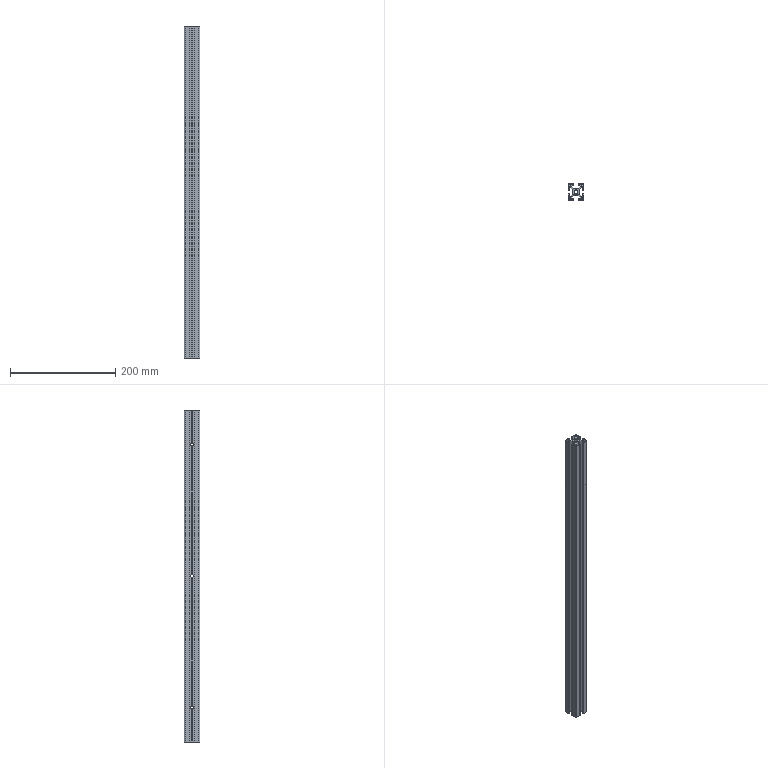Part | STEP file | SQ-8-3030W-630 Bottom_Default | 1 solid | 134 faces | box 30 x 30 x 630 mm | volume 237831 mm3 | plane 80 | cylinder 50 | cone 4 | commonest cylinder face diameters 0.6 x14 5.5 x12 4.2 x8 10 x6 4 x4 7 x4